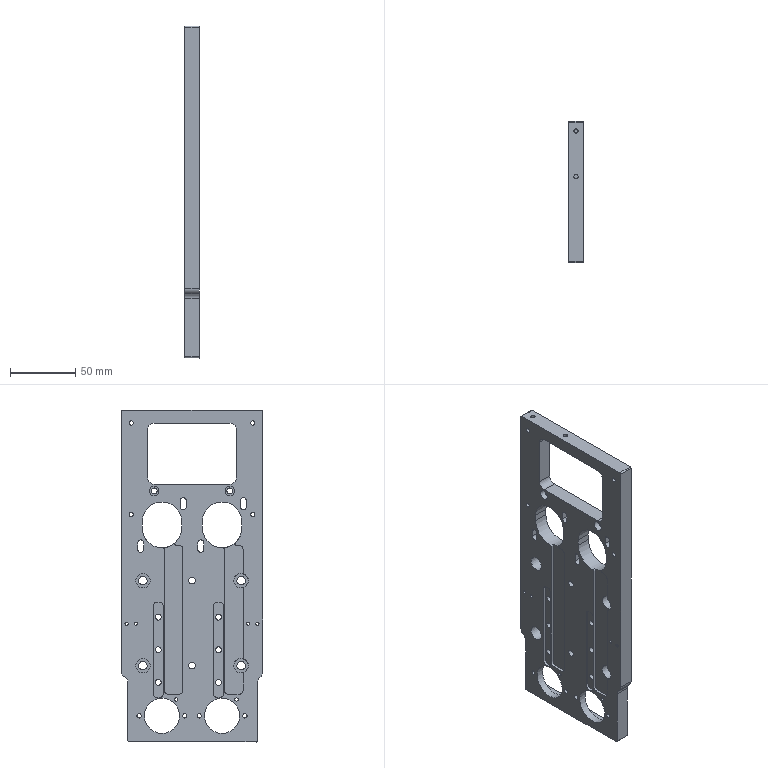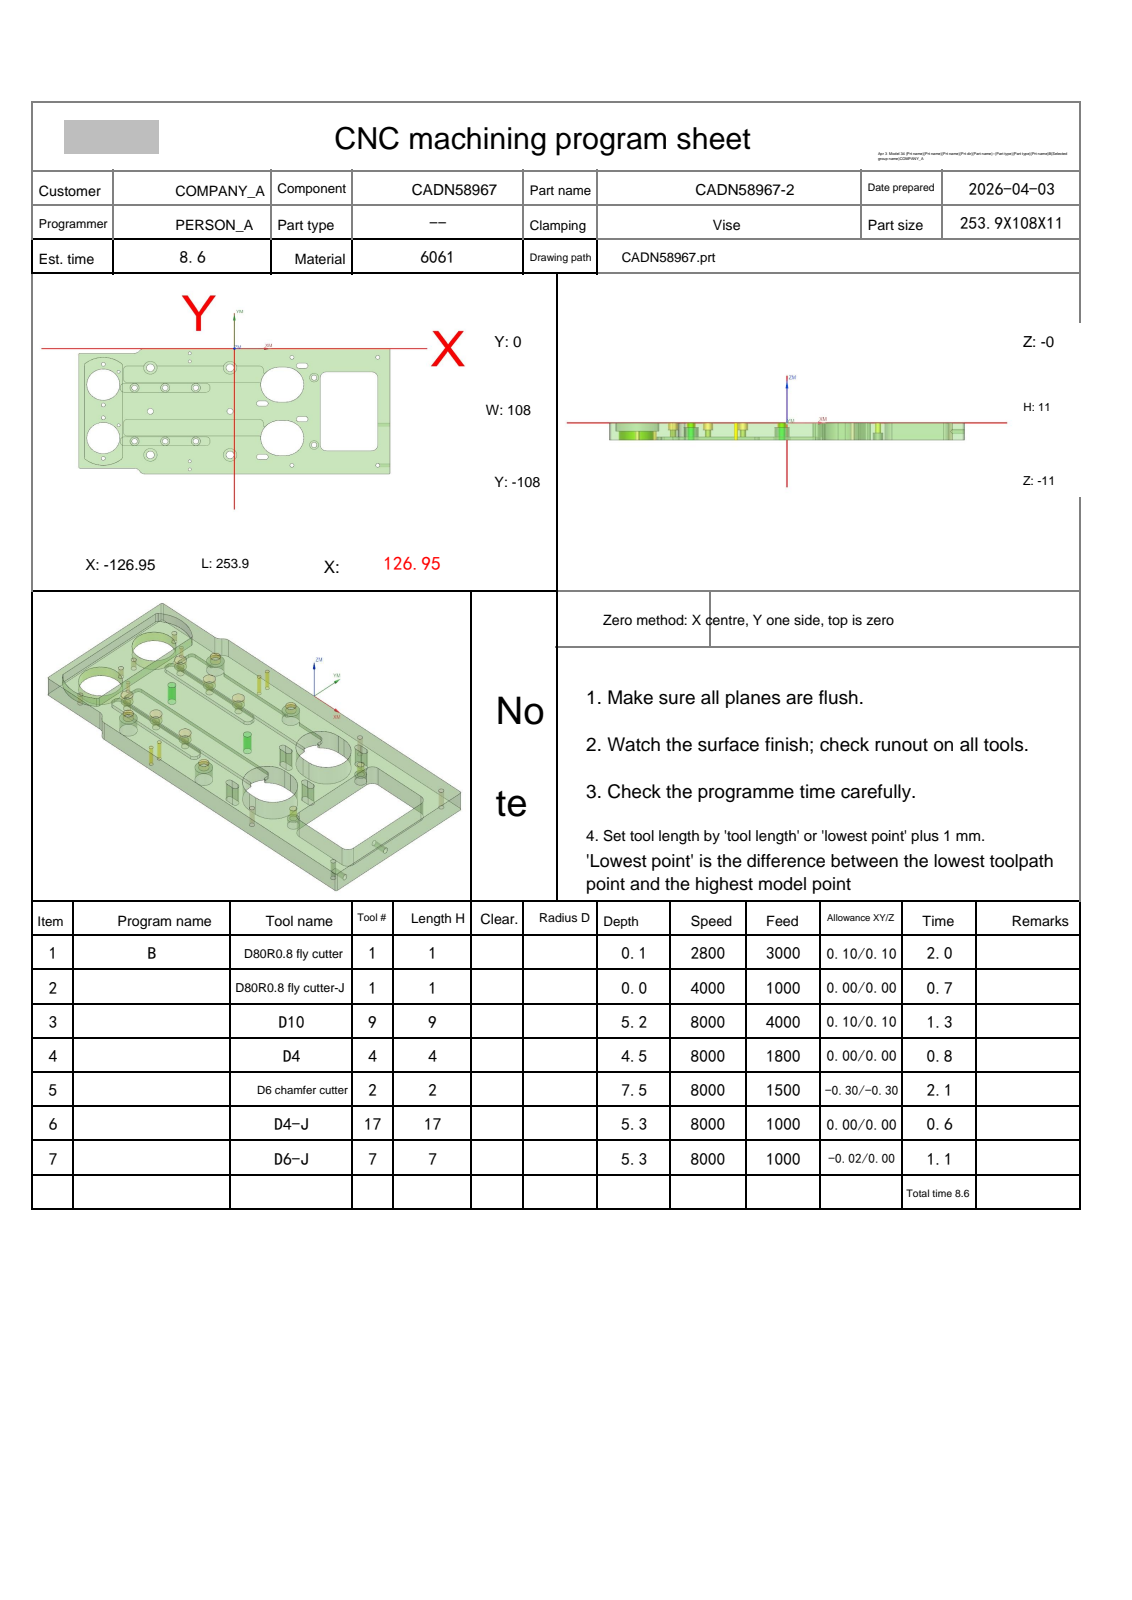NC program | NX | posted by the shop | part box 11 x 108 x 253.9 mm
Lines 3777 to 3878 of 3878:
N7 T07 M06
(D6-J  D=6. R=0. H=07 ce=0.40 di=0.00)
G00 G90 G54 X-116.05 Y-61.464 M03 S8000
G43 H07 Z13.814
M08
Z-3.3
G01 Y-54. Z-5.3 F1000.
X-119.05
Y-15.251
G02 X-118.805 Y-14.768 I.6 J-.001
X-106.95 Y-10.9 I11.855 J-16.232
X-95.095 Y-14.768 I0.0 J-20.1
X-94.85 Y-15.251 I-.355 J-.484
G01 Y-92.749
G02 X-95.095 Y-93.232 I-.6 J.001
X-106.95 Y-97.1 I-11.855 J16.232
X-118.805 Y-93.232 I0.0 J20.1
X-119.05 Y-92.749 I.355 J.484
G01 Y-52.748
G02 X-118.875 Y-52.325 I.6 J0.0
G01 X-116.225 Y-49.675
G03 X-116.05 Y-49.252 I-.425 J.424
G01 Y-16.856
G02 X-115.76 Y-16.344 I.6 J-.002
X-106.95 Y-13.9 I8.81 J-14.656
X-98.14 Y-16.344 I0.0 J-17.1
X-97.85 Y-16.856 I-.31 J-.513
G01 Y-91.144
G02 X-98.14 Y-91.656 I-.6 J.002
X-106.95 Y-94.1 I-8.81 J14.656
X-115.76 Y-91.656 I0.0 J17.1
X-116.05 Y-91.144 I.31 J.513
G01 Y-52.748
G02 X-115.875 Y-52.325 I.6 J0.0
G01 X-113.225 Y-49.675
G03 X-113.05 Y-49.252 I-.425 J.424
G01 Y-18.669
G02 X-112.696 Y-18.124 I.6 J-.002
X-106.95 Y-16.9 I5.746 J-12.876
X-101.204 Y-18.124 I0.0 J-14.1
X-100.85 Y-18.669 I-.246 J-.547
G01 Y-89.331
G02 X-101.204 Y-89.876 I-.6 J.002
X-106.95 Y-91.1 I-5.746 J12.876
X-112.696 Y-89.876 I0.0 J14.1
X-113.05 Y-89.331 I.246 J.547
G01 Y-52.748
G02 X-112.875 Y-52.325 I.6 J0.0
G01 X-110.225 Y-49.675
G03 X-110.05 Y-49.252 I-.425 J.424
G01 Y-20.8
G02 X-109.595 Y-20.22 I.6 J-.002
X-106.95 Y-19.9 I2.645 J-10.78
X-104.305 Y-20.22 I0.0 J-11.1
X-103.85 Y-20.8 I-.145 J-.582
G01 Y-87.2
G02 X-104.305 Y-87.78 I-.6 J.002
X-106.95 Y-88.1 I-2.645 J10.78
X-109.595 Y-87.78 I0.0 J11.1
X-110.05 Y-87.2 I.145 J.582
G01 Y-52.598
G02 X-109.875 Y-52.175 I.6 J0.0
G01 X-107.526 Y-49.826
G03 X-107.35 Y-49.401 I-.424 J.424
G01 Y-22.958
G02 X-106.994 Y-22.6 I.36 J-.002
G01 X-106.906
G02 X-106.55 Y-22.958 I-.004 J-.36
G01 Y-85.042
G02 X-106.906 Y-85.4 I-.36 J.002
G01 X-106.994
G02 X-107.35 Y-85.042 I.004 J.36
G01 Y-51.
Y-50.
G03 X-108.55 Y-48.8 I-1.2 J0.0
G01 Z-3.8
G00 Z13.814
G00 G90 X-117.739 Y-15.215 M03 S8000
Z13.814
Z-4.3
G01 Z-5.3 F1000.
G41 D07
X-117.856 Y-15.053
G03 X-118.828 Y-14.556 I-.972 J-.703
X-119.47 Y-14.742 I0.0 J-1.2
G01 Y-93.258
G03 X-106.95 Y-97.52 I12.52 J16.258
X-94.43 Y-93.258 I0.0 J20.52
G01 Y-14.742
G03 X-106.95 Y-10.48 I-12.52 J-16.258
X-119.47 Y-14.742 I0.0 J-20.52
G01 Y-15.142
G03 X-118.27 Y-16.342 I1.2 J0.0
G01 G40 X-118.07
Z-4.3
G00 Z13.814
M05
M09
G91 G28 Z0.0
G91 G28 Y0.0
M30
%